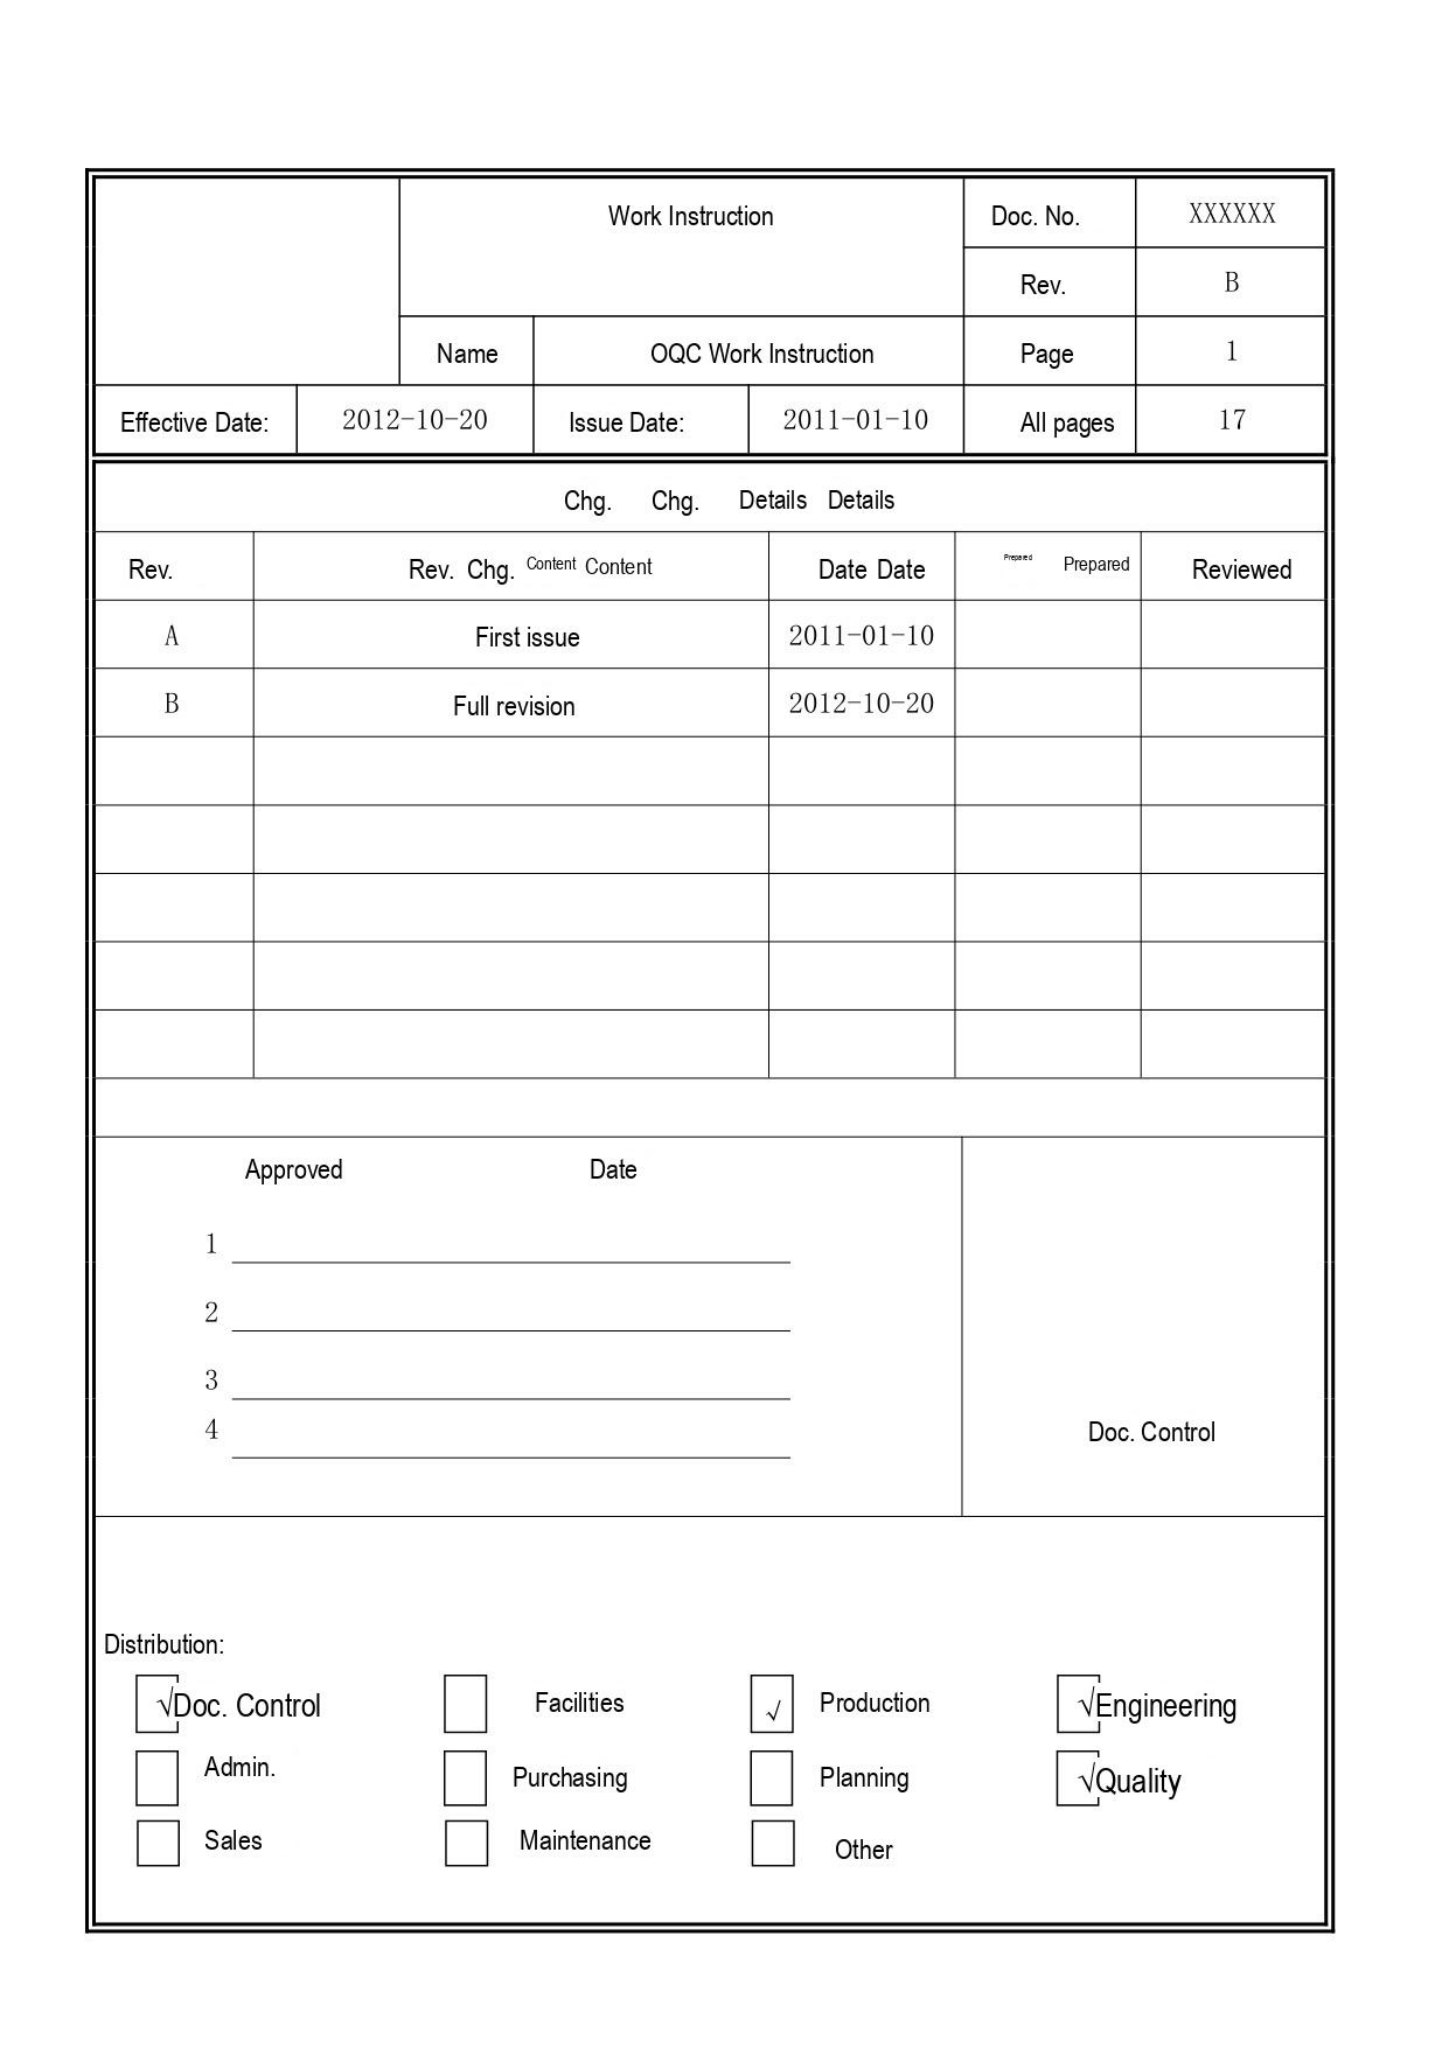| | Work Instruction | | Doc. No. | XXXXXX |
|---|---|---|---|---|
| | | | Rev. | B |
| | Name | OQC Work Instruction | Page | 1 |
| Effective Date: 2012-10-20 | | Issue Date: 2011-01-10 | All pages | 17 |

Chg. Chg. Details Details

| Rev. | Rev. Chg. Content Content | Date Date | Prepared Prepared | Reviewed |
|---|---|---|---|---|
| A | First issue | 2011-01-10 | | |
| B | Full revision | 2012-10-20 | | |
| | | | | |
| | | | | |
| | | | | |
| | | | | |
| | | | | |

Approved Date

1 ______________________

2 ______________________

3 ______________________

4 ______________________

Doc. Control

Distribution:

- [x] √Doc. Control
- [ ] Facilities
- [x] √ Production
- [x] √Engineering
- [ ] Admin.
- [ ] Purchasing
- [ ] Planning
- [x] √Quality
- [ ] Sales
- [ ] Maintenance
- [ ] Other
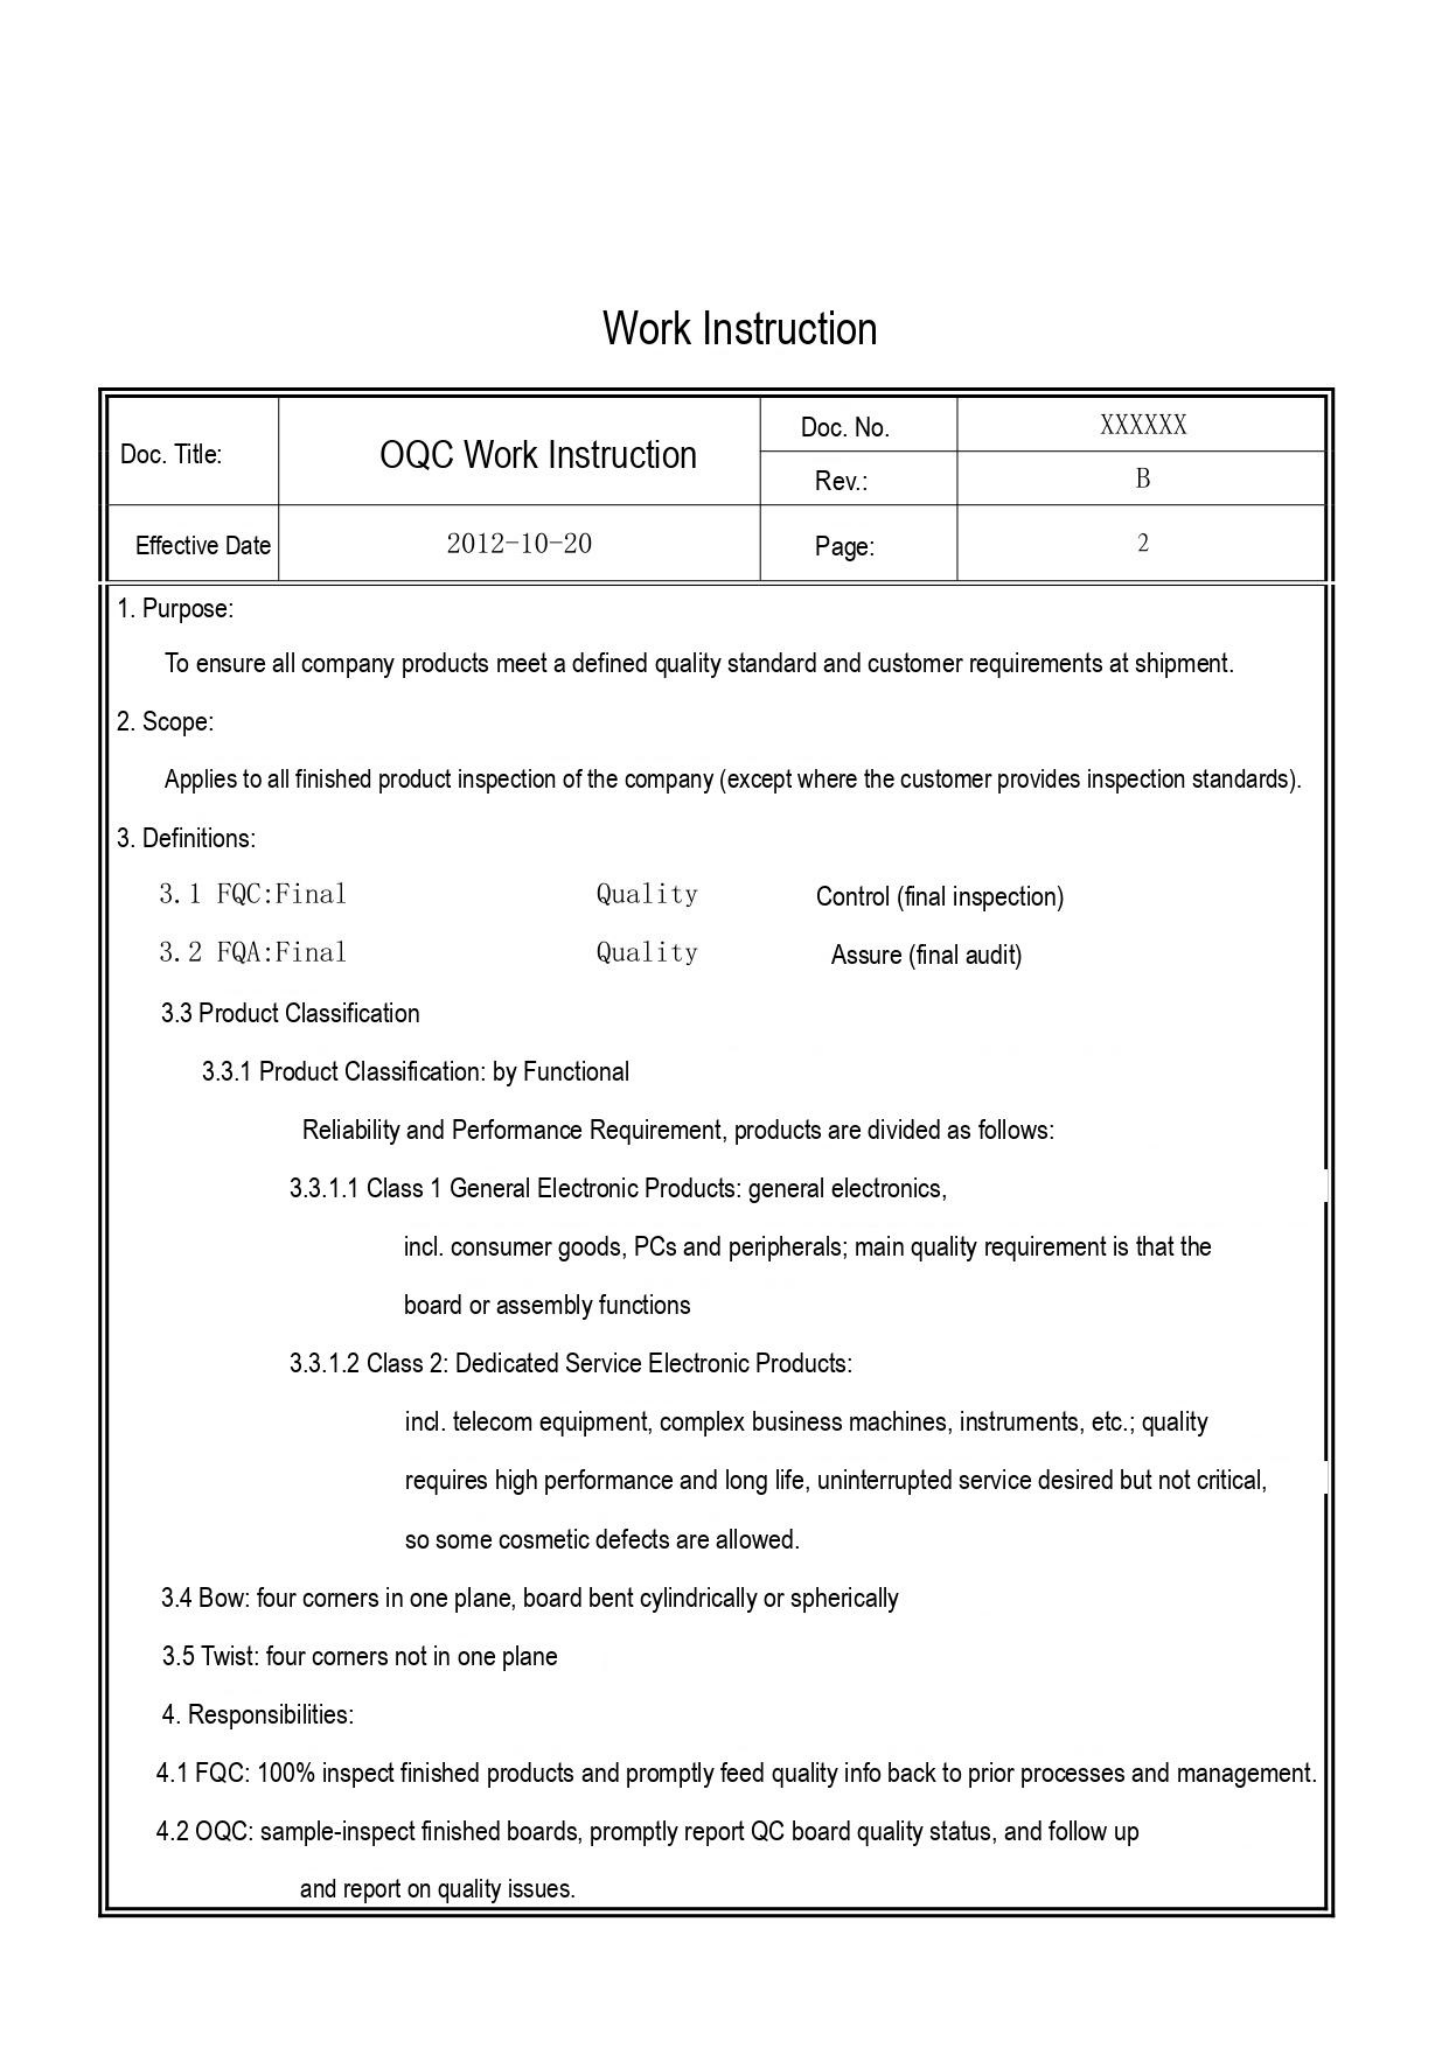Work Instruction

| Doc. Title: | OQC Work Instruction | Doc. No. | XXXXXX |
|---|---|---|---|
| | | Rev.: | B |
| Effective Date | 2012-10-20 | Page: | 2 |

1. Purpose:

To ensure all company products meet a defined quality standard and customer requirements at shipment.

2. Scope:

Applies to all finished product inspection of the company (except where the customer provides inspection standards).

3. Definitions:

3.1 FQC:Final Quality Control (final inspection)

3.2 FQA:Final Quality Assure (final audit)

3.3 Product Classification

3.3.1 Product Classification: by Functional

Reliability and Performance Requirement, products are divided as follows:

3.3.1.1 Class 1 General Electronic Products: general electronics,

incl. consumer goods, PCs and peripherals; main quality requirement is that the

board or assembly functions

3.3.1.2 Class 2: Dedicated Service Electronic Products:

incl. telecom equipment, complex business machines, instruments, etc.; quality

requires high performance and long life, uninterrupted service desired but not critical,

so some cosmetic defects are allowed.

3.4 Bow: four corners in one plane, board bent cylindrically or spherically

3.5 Twist: four corners not in one plane

4. Responsibilities:

4.1 FQC: 100% inspect finished products and promptly feed quality info back to prior processes and management.

4.2 OQC: sample-inspect finished boards, promptly report QC board quality status, and follow up

and report on quality issues.
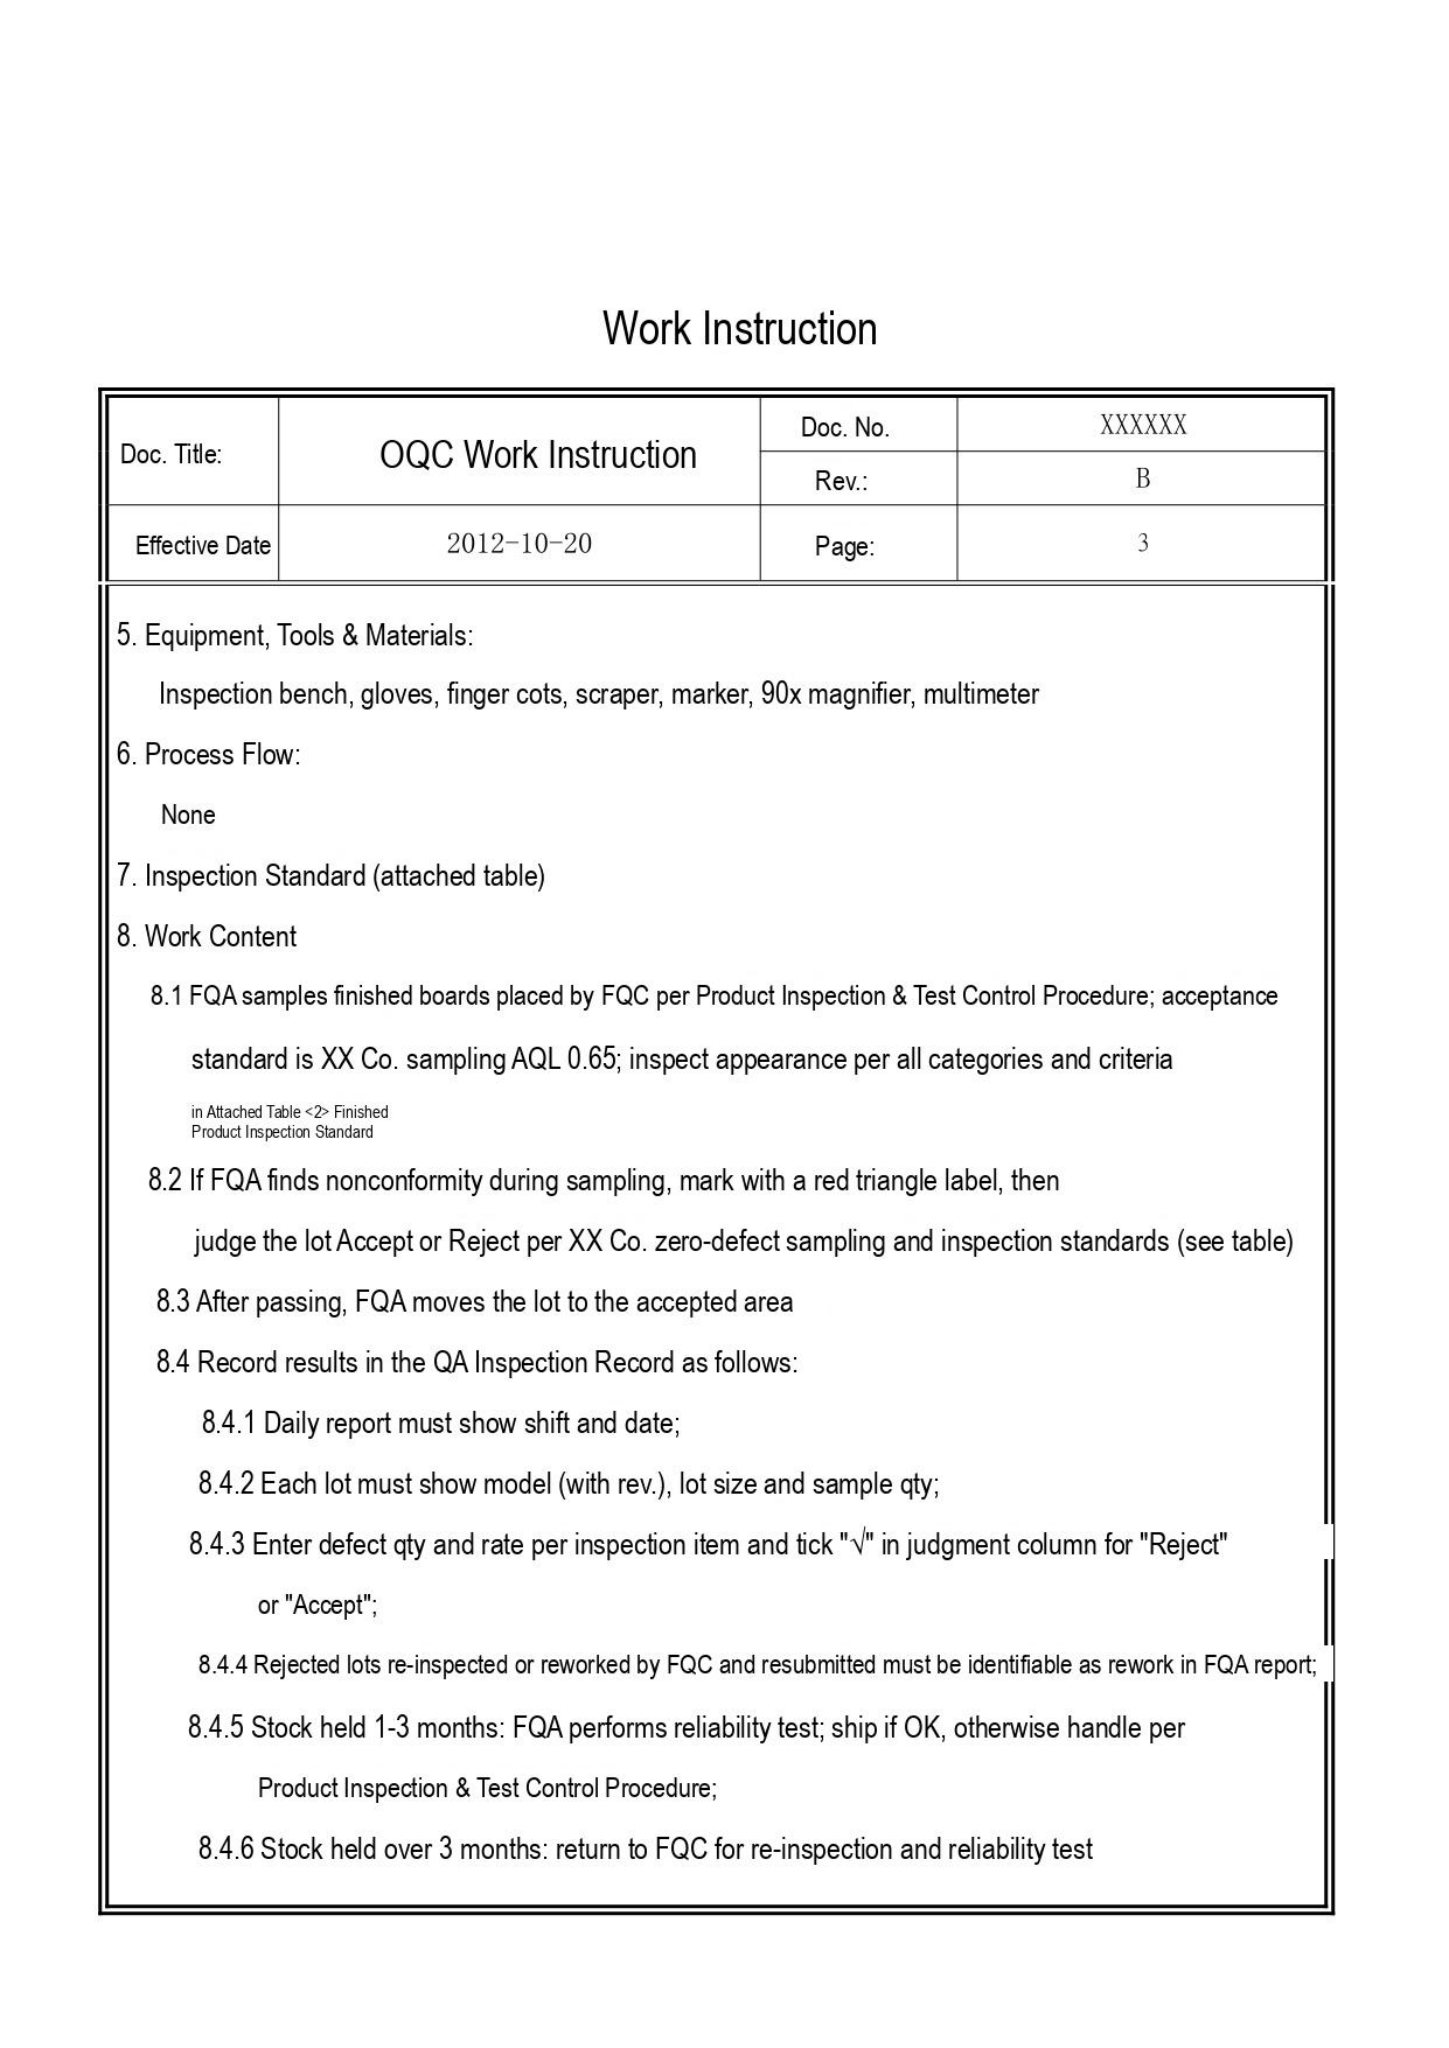Work Instruction

| Doc. Title: | OQC Work Instruction | Doc. No. | XXXXXX |
|---|---|---|---|
| | | Rev.: | B |
| Effective Date | 2012-10-20 | Page: | 3 |

5. Equipment, Tools & Materials:

Inspection bench, gloves, finger cots, scraper, marker, 90x magnifier, multimeter

6. Process Flow:

None

7. Inspection Standard (attached table)

8. Work Content

8.1 FQA samples finished boards placed by FQC per Product Inspection & Test Control Procedure; acceptance standard is XX Co. sampling AQL 0.65; inspect appearance per all categories and criteria in Attached Table <2> Finished Product Inspection Standard

8.2 If FQA finds nonconformity during sampling, mark with a red triangle label, then judge the lot Accept or Reject per XX Co. zero-defect sampling and inspection standards (see table)

8.3 After passing, FQA moves the lot to the accepted area

8.4 Record results in the QA Inspection Record as follows:

8.4.1 Daily report must show shift and date;

8.4.2 Each lot must show model (with rev.), lot size and sample qty;

8.4.3 Enter defect qty and rate per inspection item and tick "√" in judgment column for "Reject" or "Accept";

8.4.4 Rejected lots re-inspected or reworked by FQC and resubmitted must be identifiable as rework in FQA report;

8.4.5 Stock held 1-3 months: FQA performs reliability test; ship if OK, otherwise handle per Product Inspection & Test Control Procedure;

8.4.6 Stock held over 3 months: return to FQC for re-inspection and reliability test
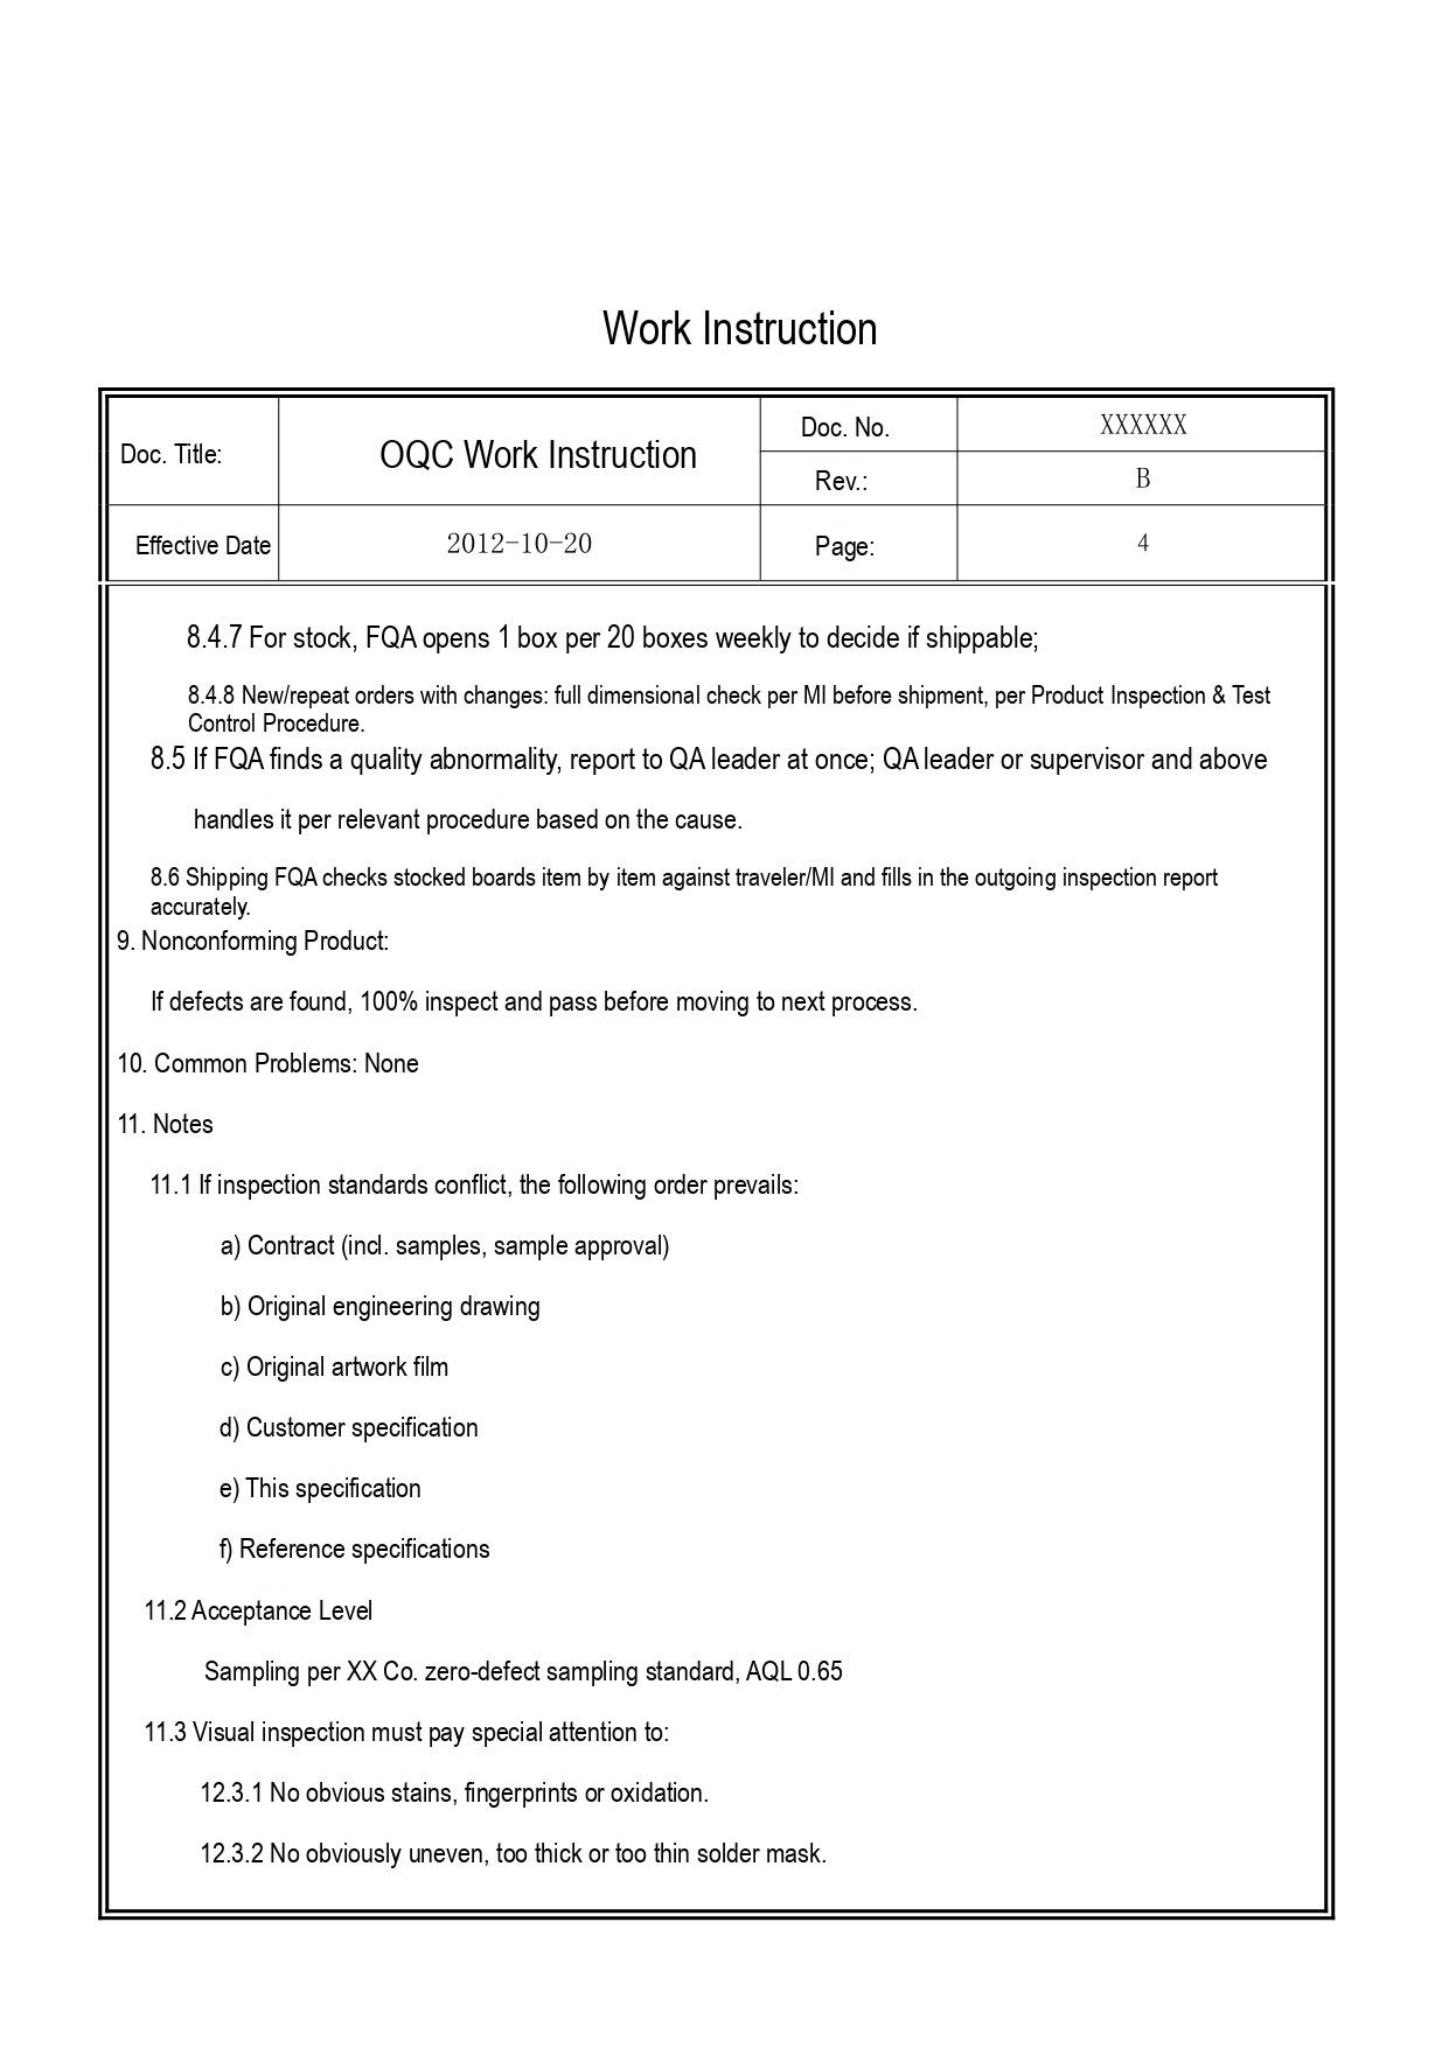Work Instruction

| Doc. Title: | OQC Work Instruction | Doc. No. | XXXXXX |
|---|---|---|---|
| | | Rev.: | B |
| Effective Date | 2012-10-20 | Page: | 4 |

8.4.7 For stock, FQA opens 1 box per 20 boxes weekly to decide if shippable;

8.4.8 New/repeat orders with changes: full dimensional check per MI before shipment, per Product Inspection & Test Control Procedure.

8.5 If FQA finds a quality abnormality, report to QA leader at once; QA leader or supervisor and above handles it per relevant procedure based on the cause.

8.6 Shipping FQA checks stocked boards item by item against traveler/MI and fills in the outgoing inspection report accurately.

9. Nonconforming Product:

If defects are found, 100% inspect and pass before moving to next process.

10. Common Problems: None

11. Notes

11.1 If inspection standards conflict, the following order prevails:

a) Contract (incl. samples, sample approval)

b) Original engineering drawing

c) Original artwork film

d) Customer specification

e) This specification

f) Reference specifications

11.2 Acceptance Level

Sampling per XX Co. zero-defect sampling standard, AQL 0.65

11.3 Visual inspection must pay special attention to:

12.3.1 No obvious stains, fingerprints or oxidation.

12.3.2 No obviously uneven, too thick or too thin solder mask.
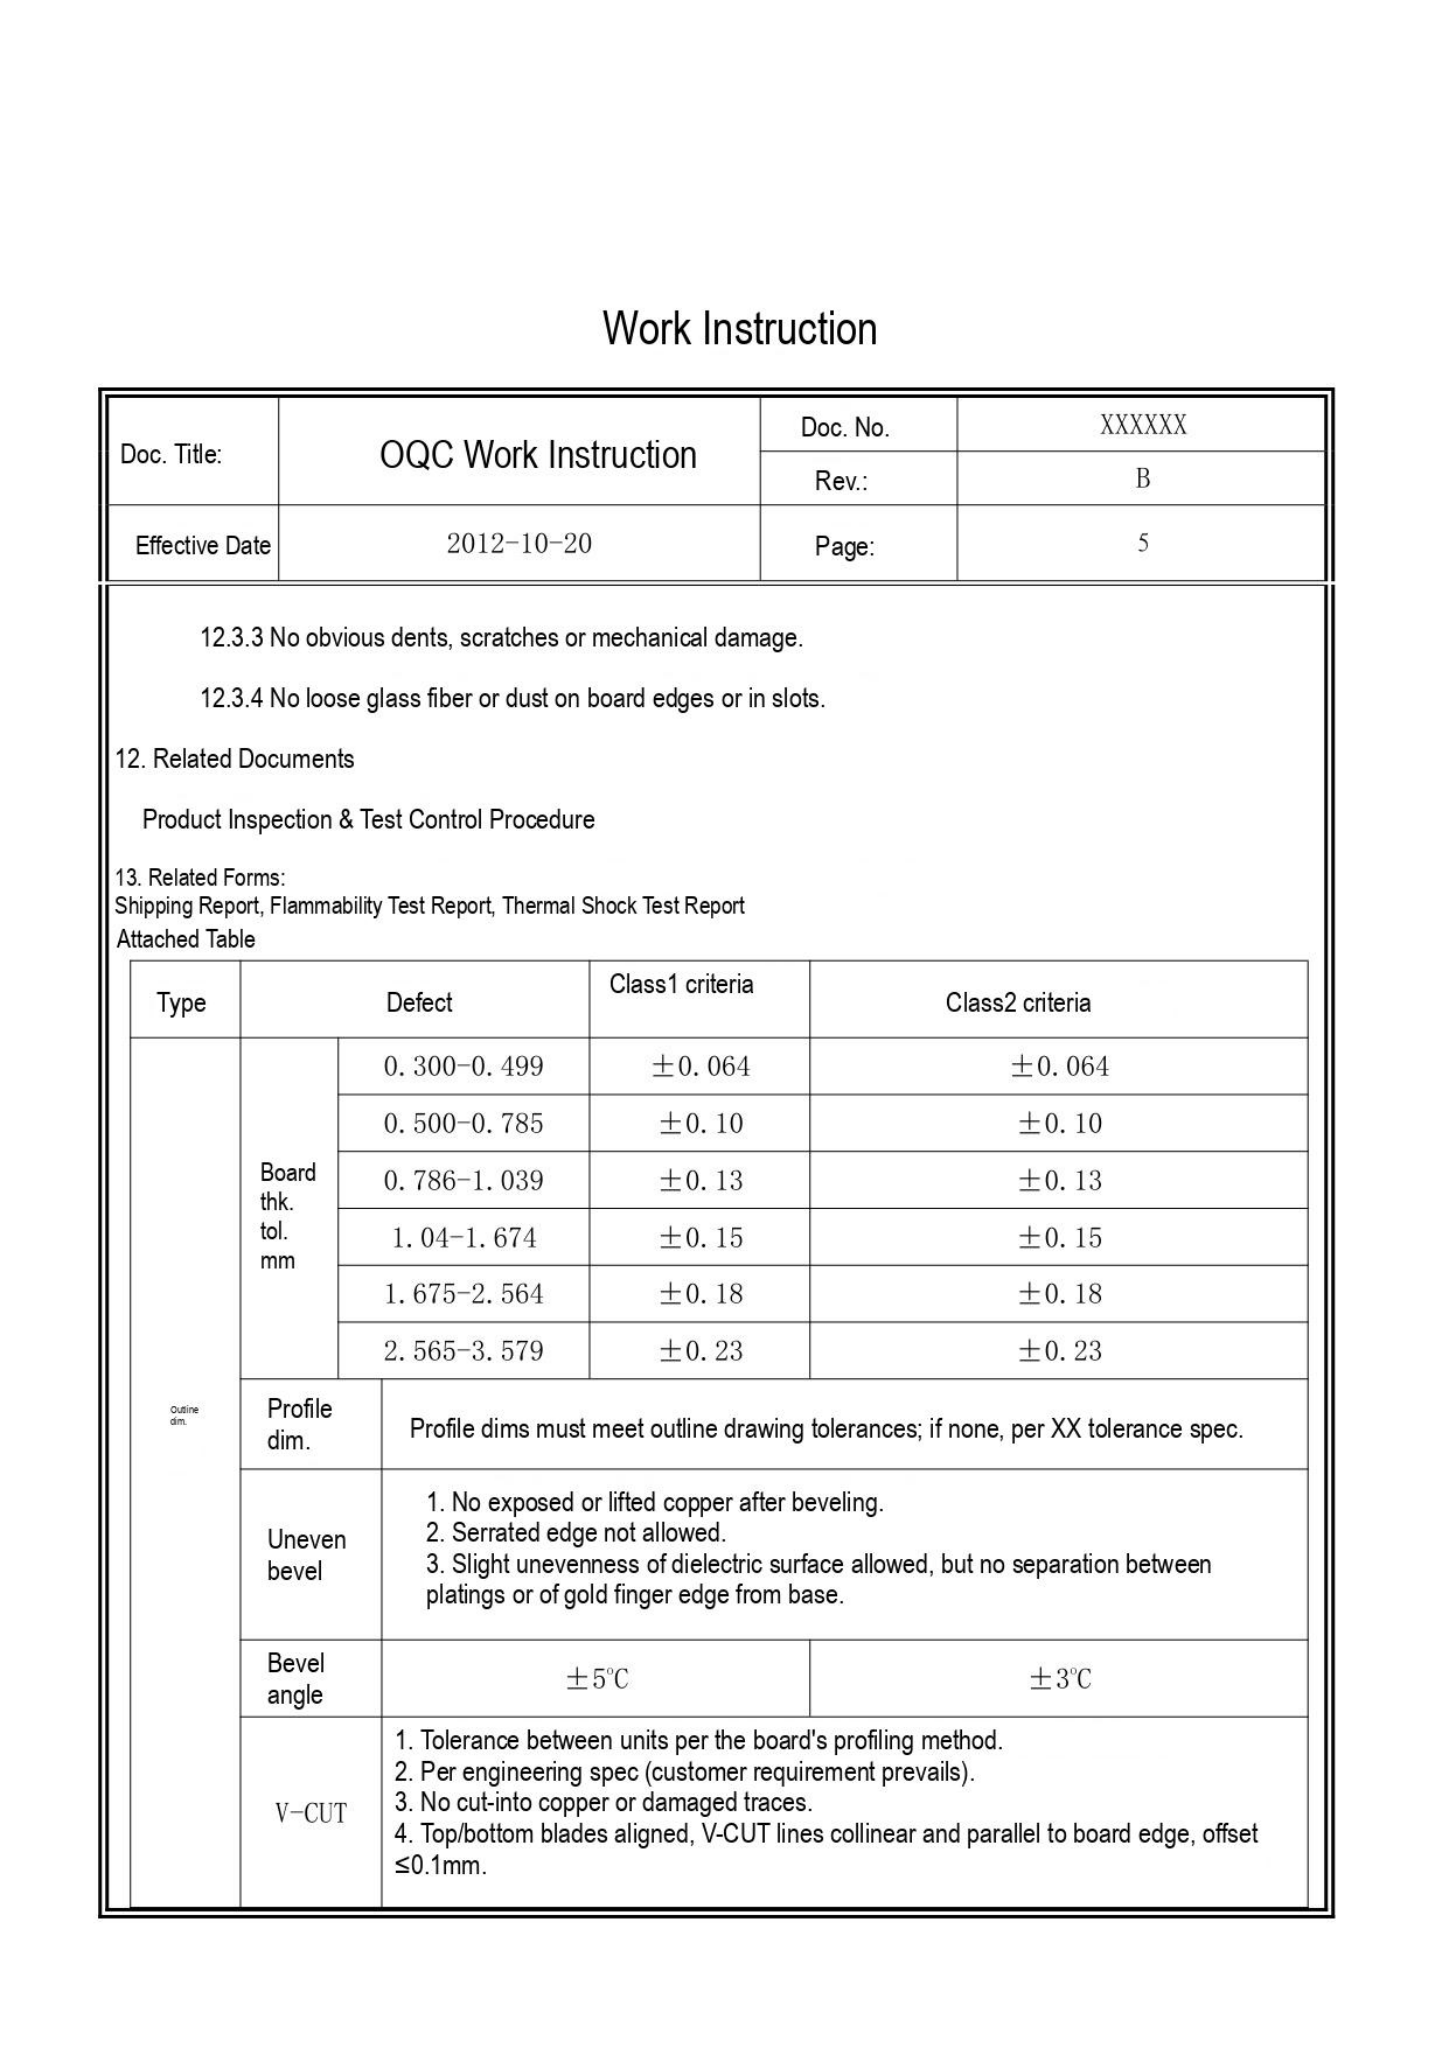# Work Instruction

| Doc. Title: | OQC Work Instruction | Doc. No. | XXXXXX |
|---|---|---|---|
| | | Rev.: | B |
| Effective Date | 2012-10-20 | Page: | 5 |

12.3.3 No obvious dents, scratches or mechanical damage.

12.3.4 No loose glass fiber or dust on board edges or in slots.

12. Related Documents

Product Inspection & Test Control Procedure

13. Related Forms:
Shipping Report, Flammability Test Report, Thermal Shock Test Report
Attached Table

| Type | Defect | | Class1 criteria | Class2 criteria |
|---|---|---|---|---|
| Outline dim. | Board thk. tol. mm | 0.300-0.499 | ±0.064 | ±0.064 |
| | | 0.500-0.785 | ±0.10 | ±0.10 |
| | | 0.786-1.039 | ±0.13 | ±0.13 |
| | | 1.04-1.674 | ±0.15 | ±0.15 |
| | | 1.675-2.564 | ±0.18 | ±0.18 |
| | | 2.565-3.579 | ±0.23 | ±0.23 |
| | Profile dim. | Profile dims must meet outline drawing tolerances; if none, per XX tolerance spec. | | |
| | Uneven bevel | 1. No exposed or lifted copper after beveling.<br>2. Serrated edge not allowed.<br>3. Slight unevenness of dielectric surface allowed, but no separation between platings or of gold finger edge from base. | | |
| | Bevel angle | ±5℃ | | ±3℃ |
| | V-CUT | 1. Tolerance between units per the board's profiling method.<br>2. Per engineering spec (customer requirement prevails).<br>3. No cut-into copper or damaged traces.<br>4. Top/bottom blades aligned, V-CUT lines collinear and parallel to board edge, offset ≤0.1mm. | | |
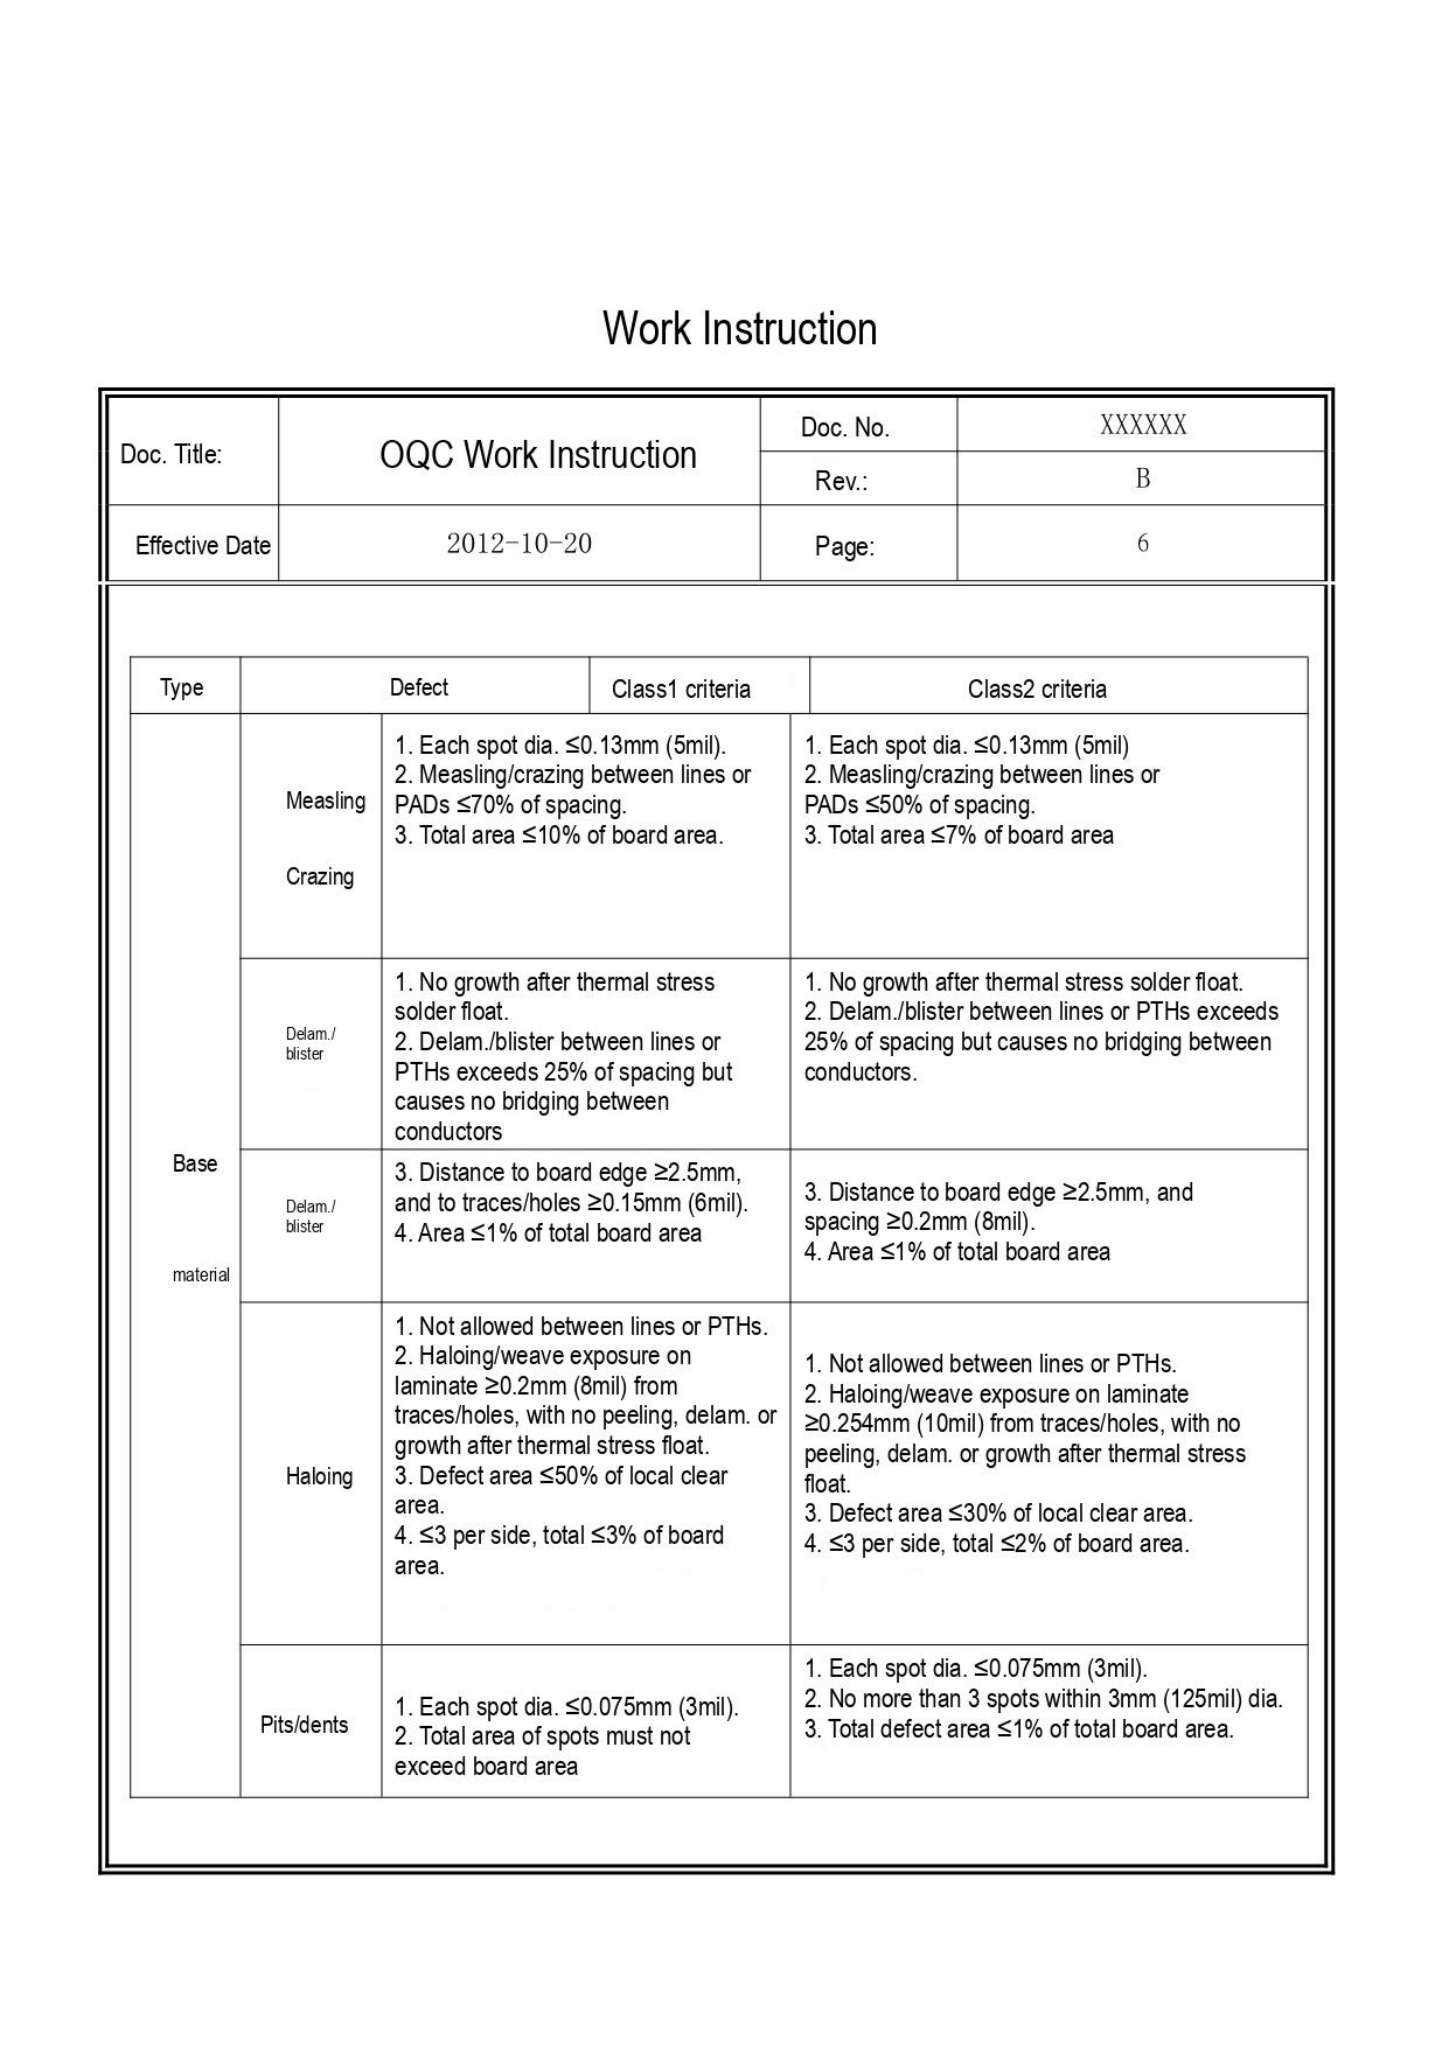Work Instruction

| Doc. Title: | OQC Work Instruction | Doc. No. | XXXXXX |
|---|---|---|---|
| | | Rev.: | B |
| Effective Date | 2012-10-20 | Page: | 6 |

| Type | Defect | Class1 criteria | Class2 criteria |
|---|---|---|---|
| Base material | Measling Crazing | 1. Each spot dia. ≤0.13mm (5mil).<br>2. Measling/crazing between lines or PADs ≤70% of spacing.<br>3. Total area ≤10% of board area. | 1. Each spot dia. ≤0.13mm (5mil)<br>2. Measling/crazing between lines or PADs ≤50% of spacing.<br>3. Total area ≤7% of board area |
| | Delam./ blister | 1. No growth after thermal stress solder float.<br>2. Delam./blister between lines or PTHs exceeds 25% of spacing but causes no bridging between conductors | 1. No growth after thermal stress solder float.<br>2. Delam./blister between lines or PTHs exceeds 25% of spacing but causes no bridging between conductors. |
| | Delam./ blister | 3. Distance to board edge ≥2.5mm, and to traces/holes ≥0.15mm (6mil).<br>4. Area ≤1% of total board area | 3. Distance to board edge ≥2.5mm, and spacing ≥0.2mm (8mil).<br>4. Area ≤1% of total board area |
| | Haloing | 1. Not allowed between lines or PTHs.<br>2. Haloing/weave exposure on laminate ≥0.2mm (8mil) from traces/holes, with no peeling, delam. or growth after thermal stress float.<br>3. Defect area ≤50% of local clear area.<br>4. ≤3 per side, total ≤3% of board area. | 1. Not allowed between lines or PTHs.<br>2. Haloing/weave exposure on laminate ≥0.254mm (10mil) from traces/holes, with no peeling, delam. or growth after thermal stress float.<br>3. Defect area ≤30% of local clear area.<br>4. ≤3 per side, total ≤2% of board area. |
| | Pits/dents | 1. Each spot dia. ≤0.075mm (3mil).<br>2. Total area of spots must not exceed board area | 1. Each spot dia. ≤0.075mm (3mil).<br>2. No more than 3 spots within 3mm (125mil) dia.<br>3. Total defect area ≤1% of total board area. |
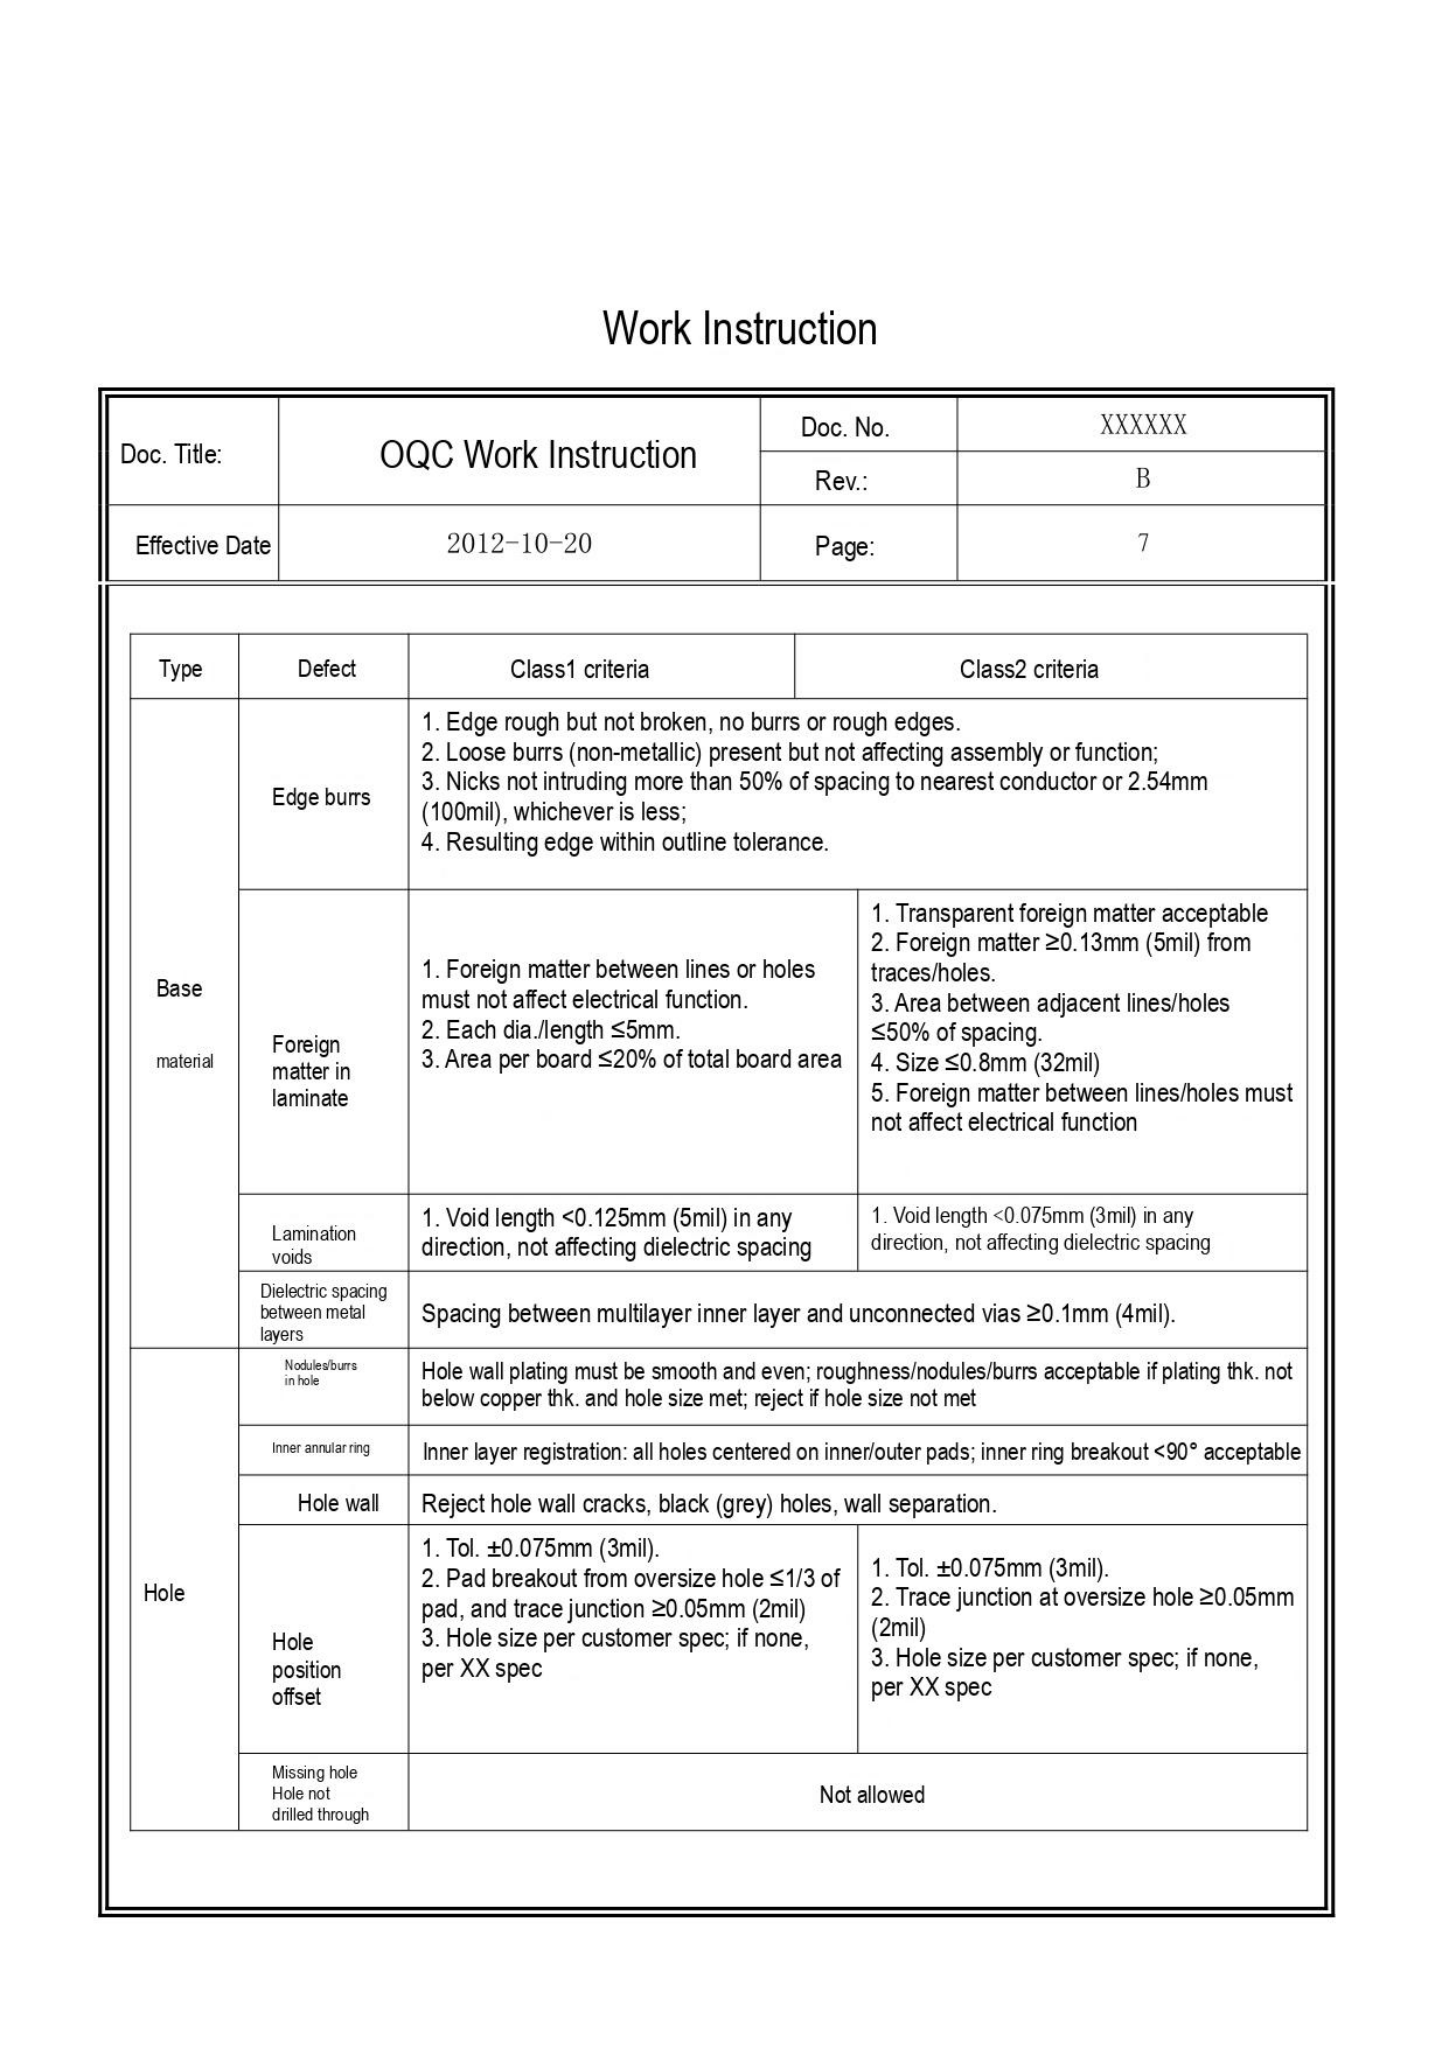Work Instruction

| Doc. Title: | OQC Work Instruction | Doc. No. | XXXXXX |
|---|---|---|---|
| | | Rev.: | B |
| Effective Date | 2012-10-20 | Page: | 7 |

| Type | Defect | Class1 criteria | Class2 criteria |
|---|---|---|---|
| Base material | Edge burrs | 1. Edge rough but not broken, no burrs or rough edges.<br>2. Loose burrs (non-metallic) present but not affecting assembly or function;<br>3. Nicks not intruding more than 50% of spacing to nearest conductor or 2.54mm (100mil), whichever is less;<br>4. Resulting edge within outline tolerance. | |
| | Foreign matter in laminate | 1. Foreign matter between lines or holes must not affect electrical function.<br>2. Each dia./length ≤5mm.<br>3. Area per board ≤20% of total board area | 1. Transparent foreign matter acceptable<br>2. Foreign matter ≥0.13mm (5mil) from traces/holes.<br>3. Area between adjacent lines/holes ≤50% of spacing.<br>4. Size ≤0.8mm (32mil)<br>5. Foreign matter between lines/holes must not affect electrical function |
| | Lamination voids | 1. Void length <0.125mm (5mil) in any direction, not affecting dielectric spacing | 1. Void length <0.075mm (3mil) in any direction, not affecting dielectric spacing |
| | Dielectric spacing between metal layers | Spacing between multilayer inner layer and unconnected vias ≥0.1mm (4mil). | |
| Hole | Nodules/burrs in hole | Hole wall plating must be smooth and even; roughness/nodules/burrs acceptable if plating thk. not below copper thk. and hole size met; reject if hole size not met | |
| | Inner annular ring | Inner layer registration: all holes centered on inner/outer pads; inner ring breakout <90° acceptable | |
| | Hole wall | Reject hole wall cracks, black (grey) holes, wall separation. | |
| | Hole position offset | 1. Tol. ±0.075mm (3mil).<br>2. Pad breakout from oversize hole ≤1/3 of pad, and trace junction ≥0.05mm (2mil)<br>3. Hole size per customer spec; if none, per XX spec | 1. Tol. ±0.075mm (3mil).<br>2. Trace junction at oversize hole ≥0.05mm (2mil)<br>3. Hole size per customer spec; if none, per XX spec |
| | Missing hole<br>Hole not drilled through | Not allowed | |